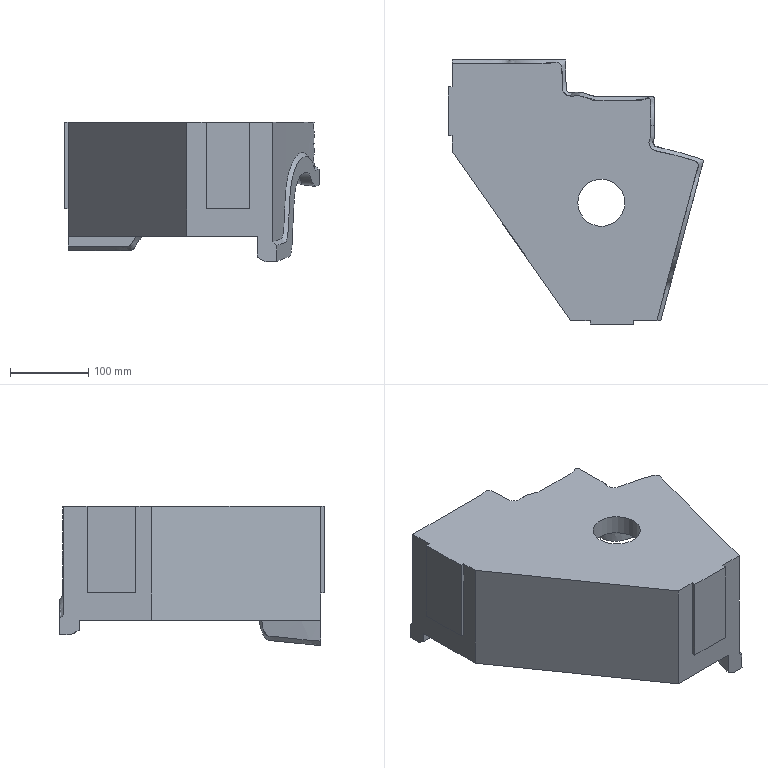Part | NX | features solid 2 | 1 solid | 54 faces | box 325.443 x 337.546 x 177.389 mm | volume 4296999 mm3 | plane 32 | spline 15 | cylinder 7 | commonest cylinder face diameters 30 x6 60 x1